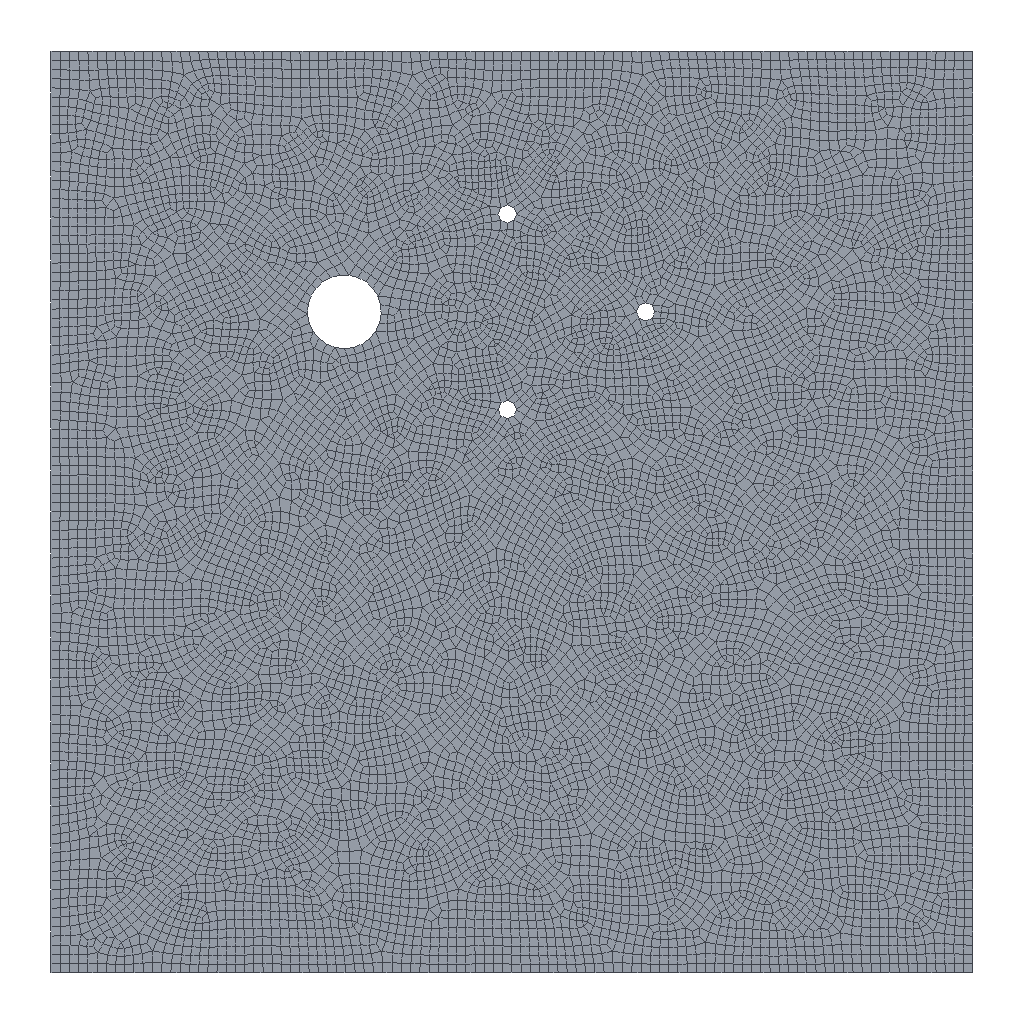Simulation study | abaqus
Abaqus input file, long lists of numbers shortened:
*Heading
** Job name: Job-1 Model name: Model-1
** Generated by: Abaqus/CAE 2020
*Preprint, echo=NO, model=NO, history=NO, contact=NO
**
** PARTS
**
*Part, name=Part-1
*Node
      1,         980.,           0.
      2,         960.,           0.
** (12449 more lines like these left out)
*Element, type=CPS3
  1, 11426,  8633, 11383
  2,  7287,  2273,  7250
** (403 more lines like these left out)
*Element, type=CPS4R
  406,  2392,     1,  2839,  2635
  407,  2392,  2635,  2599,    48
** (12025 more lines like these left out)
*Nset, nset=Set-2, generate
     1,  12451,      1
*Elset, elset=Set-2, generate
     1,  12432,      1
** Section: Section-1
*Solid Section, elset=Set-2, material=Material-1
,
*End Part
**
**
** ASSEMBLY
**
*Assembly, name=Assembly
**
*Instance, name=Part-1-1, part=Part-1
*End Instance
**
*Nset, nset=Set-1, instance=Part-1-1
   97,   98,   99,  100,  101,  102,  103,  104,  105,  106,  107,  108,  109,  110,  111,  112
  113,  114,  115,  116,  117,  118,  119,  120,  121,  122,  123,  124,  125,  126,  127,  128
** (5 more lines like these left out)
*Elset, elset=Set-1, instance=Part-1-1
  454,  504,  505,  506,  507,  593,  639,  683,  726,  775,  825,  929,  930,  931, 1013, 1014
 1059, 1060, 1103, 1149, 1195, 1244, 1290, 1391, 1392, 1393, 1394, 1547, 1548, 1597, 1643, 1692
** (5 more lines like these left out)
*Nset, nset=Set-2, instance=Part-1-1
 49,
*Nset, nset=Set-3, instance=Part-1-1
 48,
*Elset, elset=_Surf-1_S1, internal, instance=Part-1-1
  406,  456,  547,  594,  641,  685,  728,  777,  778,  827,  828,  853,  854,  867,  881,  967
 1015, 1061, 1104, 1151, 1197, 1246, 1292, 1293, 1343, 1345, 1418, 1419, 1443, 1444, 1467, 1491
** (4 more lines like these left out)
*Elset, elset=_Surf-1_S4, internal, instance=Part-1-1
 407,
*Elset, elset=_Surf-1_S3, internal, instance=Part-1-1
  729, 1247, 1489, 1646, 2091, 4577, 4578, 4850
*Surface, type=ELEMENT, name=Surf-1
_Surf-1_S1, S1
_Surf-1_S4, S4
_Surf-1_S3, S3
*Nset, nset="_T-Datum csys-1", internal
Set-2,
*Transform, nset="_T-Datum csys-1"
0.7071, -0.7071,           0., -0.7071, -0.7071,           0.
*Nset, nset="_T-Datum csys-2", internal
Set-3,
*Transform, nset="_T-Datum csys-2"
-0.7071, -0.7071,           0., -0.7071, 0.7071,           0.
*End Assembly
**
** MATERIALS
**
*Material, name=Material-1
*Density
 7.8e-09,
*Elastic
210000., 0.3
*Plastic
300.,    0.
320., 0.015
** ----------------------------------------------------------------
**
** STEP: Step-1
**
*Step, name=Step-1, nlgeom=YES, inc=1000
*Static
0.01, 1., 1e-05, 1.
**
** BOUNDARY CONDITIONS
**
** Name: BC-1 Type: 对称/反对称/完全固定
*Boundary
Set-1, ENCASTRE
**
** LOADS
**
** Name: Load-2   Type: Concentrated force
*Cload
Set-2, 1, -460.
** Name: Load-3   Type: Concentrated force
*Cload
Set-3, 1, -460.
** Name: Load-p   Type: Pressure
*Dsload
Surf-1, P, 100.
**
** OUTPUT REQUESTS
**
*Restart, write, frequency=0
**
** FIELD OUTPUT: F-Output-1
**
*Output, field
*Node Output
CF, RF, RM, RT, U, V
*Element Output, directions=YES
E, LE, MISES, MISESMAX, MISESONLY, PE, PEEQ, PEEQMAX, PEEQT, PEMAG, PRESSONLY, S, SEQUT, SSAVG, YIELDPOT
*Contact Output
CDISP, CSTRESS
**
** HISTORY OUTPUT: H-Output-1
**
*Output, history, variable=PRESELECT
*End Step